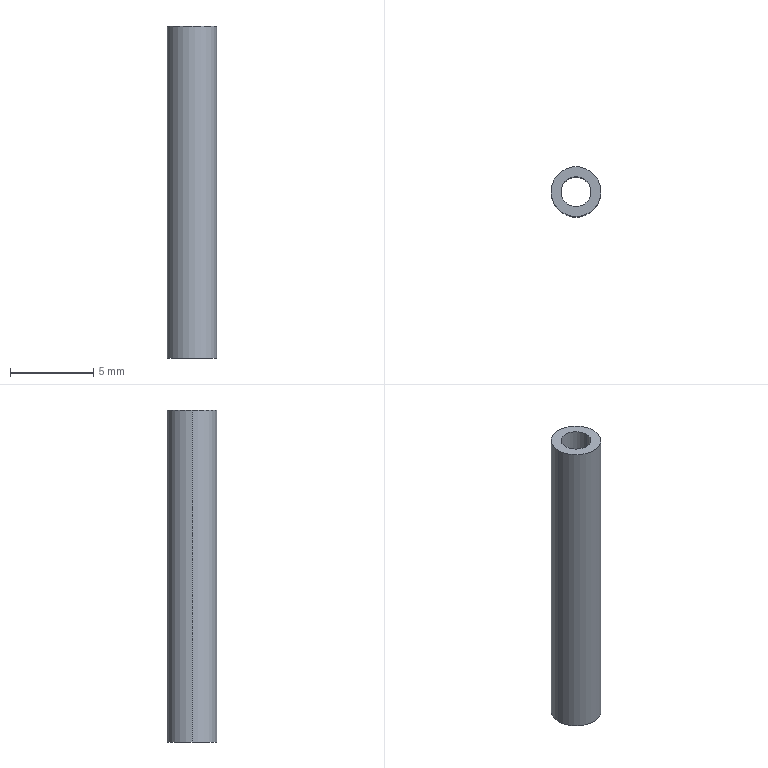Part | SolidWorks | features Extrusion 1 | 1 solid | 6 faces | box 3 x 3 x 20 mm | volume 90.478 mm3 | cylinder 4 | plane 2 | commonest cylinder face diameters 1.8 x2 3 x2
STEP:
#1=CARTESIAN_POINT('',(-0.9,0.,20.));
#2=VERTEX_POINT('',#1);
#3=CARTESIAN_POINT('',(0.9,0.,20.));
#4=VERTEX_POINT('',#3);
#5=CARTESIAN_POINT('',(0.,0.,20.));
#6=DIRECTION('',(0.,0.,1.));
#7=DIRECTION('',(1.,0.,0.));
#8=AXIS2_PLACEMENT_3D('',#5,#6,#7);
#9=CIRCLE('',#8,0.9);
#10=EDGE_CURVE('',#2,#4,#9,.T.);
#11=ORIENTED_EDGE('',*,*,#10,.T.);
#12=CARTESIAN_POINT('',(0.9,0.,0.));
#13=VERTEX_POINT('',#12);
#14=CARTESIAN_POINT('',(0.9,0.,20.));
#15=DIRECTION('',(0.,0.,-1.));
#16=VECTOR('',#15,1000.);
#17=LINE('',#14,#16);
#18=EDGE_CURVE('',#4,#13,#17,.T.);
#19=ORIENTED_EDGE('',*,*,#18,.T.);
#20=CARTESIAN_POINT('',(-0.9,0.,0.));
#21=VERTEX_POINT('',#20);
#22=CARTESIAN_POINT('',(0.,0.,0.));
#23=DIRECTION('',(0.,0.,1.));
#24=DIRECTION('',(1.,0.,0.));
#25=AXIS2_PLACEMENT_3D('',#22,#23,#24);
#26=CIRCLE('',#25,0.9);
#27=EDGE_CURVE('',#21,#13,#26,.T.);
#28=ORIENTED_EDGE('',*,*,#27,.F.);
#29=CARTESIAN_POINT('',(-0.9,0.,20.));
#30=DIRECTION('',(0.,0.,-1.));
#31=VECTOR('',#30,1000.);
#32=LINE('',#29,#31);
#33=EDGE_CURVE('',#2,#21,#32,.T.);
#34=ORIENTED_EDGE('',*,*,#33,.F.);
#35=EDGE_LOOP('',(#11,#19,#28,#34));
#36=FACE_OUTER_BOUND('',#35,.T.);
#37=CARTESIAN_POINT('',(0.,0.,20.));
#38=DIRECTION('',(0.,0.,-1.));
#39=DIRECTION('',(-1.,0.,0.));
#40=AXIS2_PLACEMENT_3D('',#37,#38,#39);
#41=CYLINDRICAL_SURFACE('',#40,0.9);
#42=ADVANCED_FACE('',(#36),#41,.F.);
#43=CARTESIAN_POINT('',(1.5,0.,20.));
#44=VERTEX_POINT('',#43);
#45=CARTESIAN_POINT('',(-1.5,0.,20.));
#46=VERTEX_POINT('',#45);
#47=CARTESIAN_POINT('',(0.,0.,20.));
#48=DIRECTION('',(0.,0.,1.));
#49=DIRECTION('',(1.,0.,0.));
#50=AXIS2_PLACEMENT_3D('',#47,#48,#49);
#51=CIRCLE('',#50,1.5);
#52=EDGE_CURVE('',#44,#46,#51,.T.);
#53=ORIENTED_EDGE('',*,*,#52,.F.);
#54=CARTESIAN_POINT('',(1.5,0.,0.));
#55=VERTEX_POINT('',#54);
#56=CARTESIAN_POINT('',(1.5,0.,20.));
#57=DIRECTION('',(0.,0.,-1.));
#58=VECTOR('',#57,1000.);
#59=LINE('',#56,#58);
#60=EDGE_CURVE('',#44,#55,#59,.T.);
#61=ORIENTED_EDGE('',*,*,#60,.T.);
#62=CARTESIAN_POINT('',(-1.5,0.,0.));
#63=VERTEX_POINT('',#62);
#64=CARTESIAN_POINT('',(0.,0.,0.));
#65=DIRECTION('',(0.,0.,1.));
#66=DIRECTION('',(1.,0.,0.));
#67=AXIS2_PLACEMENT_3D('',#64,#65,#66);
#68=CIRCLE('',#67,1.5);
#69=EDGE_CURVE('',#55,#63,#68,.T.);
#70=ORIENTED_EDGE('',*,*,#69,.T.);
#71=CARTESIAN_POINT('',(-1.5,0.,20.));
#72=DIRECTION('',(0.,0.,-1.));
#73=VECTOR('',#72,1000.);
#74=LINE('',#71,#73);
#75=EDGE_CURVE('',#46,#63,#74,.T.);
#76=ORIENTED_EDGE('',*,*,#75,.F.);
#77=EDGE_LOOP('',(#53,#61,#70,#76));
#78=FACE_OUTER_BOUND('',#77,.T.);
#79=CARTESIAN_POINT('',(0.,0.,20.));
#80=DIRECTION('',(0.,0.,-1.));
#81=DIRECTION('',(-1.,0.,0.));
#82=AXIS2_PLACEMENT_3D('',#79,#80,#81);
#83=CYLINDRICAL_SURFACE('',#82,1.5);
#84=ADVANCED_FACE('',(#78),#83,.T.);
#85=CARTESIAN_POINT('',(0.,0.,20.));
#86=DIRECTION('',(0.,0.,1.));
#87=DIRECTION('',(1.,0.,0.));
#88=AXIS2_PLACEMENT_3D('',#85,#86,#87);
#89=CIRCLE('',#88,1.5);
#90=EDGE_CURVE('',#46,#44,#89,.T.);
#91=ORIENTED_EDGE('',*,*,#90,.T.);
#92=ORIENTED_EDGE('',*,*,#52,.T.);
#93=EDGE_LOOP('',(#91,#92));
#94=FACE_OUTER_BOUND('',#93,.T.);
#95=ORIENTED_EDGE('',*,*,#10,.F.);
#96=CARTESIAN_POINT('',(0.,0.,20.));
#97=DIRECTION('',(0.,0.,1.));
#98=DIRECTION('',(1.,0.,0.));
#99=AXIS2_PLACEMENT_3D('',#96,#97,#98);
#100=CIRCLE('',#99,0.9);
#101=EDGE_CURVE('',#4,#2,#100,.T.);
#102=ORIENTED_EDGE('',*,*,#101,.F.);
#103=EDGE_LOOP('',(#95,#102));
#104=FACE_BOUND('',#103,.T.);
#105=CARTESIAN_POINT('',(0.,0.,20.));
#106=DIRECTION('',(0.,0.,1.));
#107=DIRECTION('',(1.,0.,0.));
#108=AXIS2_PLACEMENT_3D('',#105,#106,#107);
#109=PLANE('',#108);
#110=ADVANCED_FACE('',(#94,#104),#109,.T.);
#111=CARTESIAN_POINT('',(0.,0.,0.));
#112=DIRECTION('',(0.,0.,1.));
#113=DIRECTION('',(1.,0.,0.));
#114=AXIS2_PLACEMENT_3D('',#111,#112,#113);
#115=CIRCLE('',#114,1.5);
#116=EDGE_CURVE('',#63,#55,#115,.T.);
#117=ORIENTED_EDGE('',*,*,#116,.F.);
#118=ORIENTED_EDGE('',*,*,#69,.F.);
#119=EDGE_LOOP('',(#117,#118));
#120=FACE_OUTER_BOUND('',#119,.T.);
#121=ORIENTED_EDGE('',*,*,#27,.T.);
#122=CARTESIAN_POINT('',(0.,0.,0.));
#123=DIRECTION('',(0.,0.,1.));
#124=DIRECTION('',(1.,0.,0.));
#125=AXIS2_PLACEMENT_3D('',#122,#123,#124);
#126=CIRCLE('',#125,0.9);
#127=EDGE_CURVE('',#13,#21,#126,.T.);
#128=ORIENTED_EDGE('',*,*,#127,.T.);
#129=EDGE_LOOP('',(#121,#128));
#130=FACE_BOUND('',#129,.T.);
#131=CARTESIAN_POINT('',(0.,0.,0.));
#132=DIRECTION('',(0.,0.,1.));
#133=DIRECTION('',(1.,0.,0.));
#134=AXIS2_PLACEMENT_3D('',#131,#132,#133);
#135=PLANE('',#134);
#136=ADVANCED_FACE('',(#120,#130),#135,.F.);
#137=ORIENTED_EDGE('',*,*,#60,.F.);
#138=ORIENTED_EDGE('',*,*,#90,.F.);
#139=ORIENTED_EDGE('',*,*,#75,.T.);
#140=ORIENTED_EDGE('',*,*,#116,.T.);
#141=EDGE_LOOP('',(#137,#138,#139,#140));
#142=FACE_OUTER_BOUND('',#141,.T.);
#143=CARTESIAN_POINT('',(0.,0.,20.));
#144=DIRECTION('',(0.,0.,-1.));
#145=DIRECTION('',(-1.,0.,0.));
#146=AXIS2_PLACEMENT_3D('',#143,#144,#145);
#147=CYLINDRICAL_SURFACE('',#146,1.5);
#148=ADVANCED_FACE('',(#142),#147,.T.);
#149=ORIENTED_EDGE('',*,*,#18,.F.);
#150=ORIENTED_EDGE('',*,*,#101,.T.);
#151=ORIENTED_EDGE('',*,*,#33,.T.);
#152=ORIENTED_EDGE('',*,*,#127,.F.);
#153=EDGE_LOOP('',(#149,#150,#151,#152));
#154=FACE_OUTER_BOUND('',#153,.T.);
#155=CARTESIAN_POINT('',(0.,0.,20.));
#156=DIRECTION('',(0.,0.,-1.));
#157=DIRECTION('',(-1.,0.,0.));
#158=AXIS2_PLACEMENT_3D('',#155,#156,#157);
#159=CYLINDRICAL_SURFACE('',#158,0.9);
#160=ADVANCED_FACE('',(#154),#159,.F.);
#161=CLOSED_SHELL('',(#42,#84,#110,#136,#148,#160));
#162=MANIFOLD_SOLID_BREP('',#161);
#163=CARTESIAN_POINT('',(0.,0.,0.));
#164=DIRECTION('',(0.,0.,1.));
#165=DIRECTION('',(1.,0.,0.));
#166=AXIS2_PLACEMENT_3D('',#163,#164,#165);
#167=(LENGTH_UNIT()NAMED_UNIT(*)SI_UNIT(.MILLI.,.METRE.));
#168=UNCERTAINTY_MEASURE_WITH_UNIT(LENGTH_MEASURE(0.00001),#167,'','');
#169=(NAMED_UNIT(*)PLANE_ANGLE_UNIT()SI_UNIT($,.RADIAN.));
#170=(NAMED_UNIT(*)SI_UNIT($,.STERADIAN.)SOLID_ANGLE_UNIT());
#171=(GEOMETRIC_REPRESENTATION_CONTEXT(3)GLOBAL_UNCERTAINTY_ASSIGNED_CONTEXT((#168))GLOBAL_UNIT_ASSIGNED_CONTEXT((#167,#169,#170))REPRESENTATION_CONTEXT('',''));
#172=ADVANCED_BREP_SHAPE_REPRESENTATION('',(#162,#166),#171);